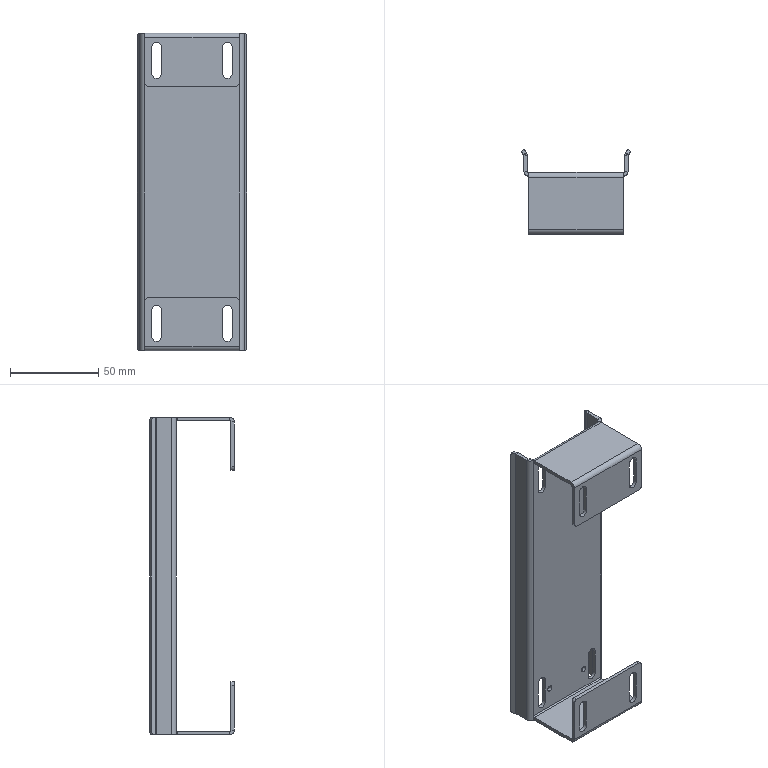Part | STEP file | 1 solid | 126 faces | box 61.928 x 48 x 180 mm | volume 40990 mm3 | plane 74 | cylinder 52 | commonest cylinder face diameters 5.5 x24 1.473 x8 4 x8 5.473 x8 3.3 x4